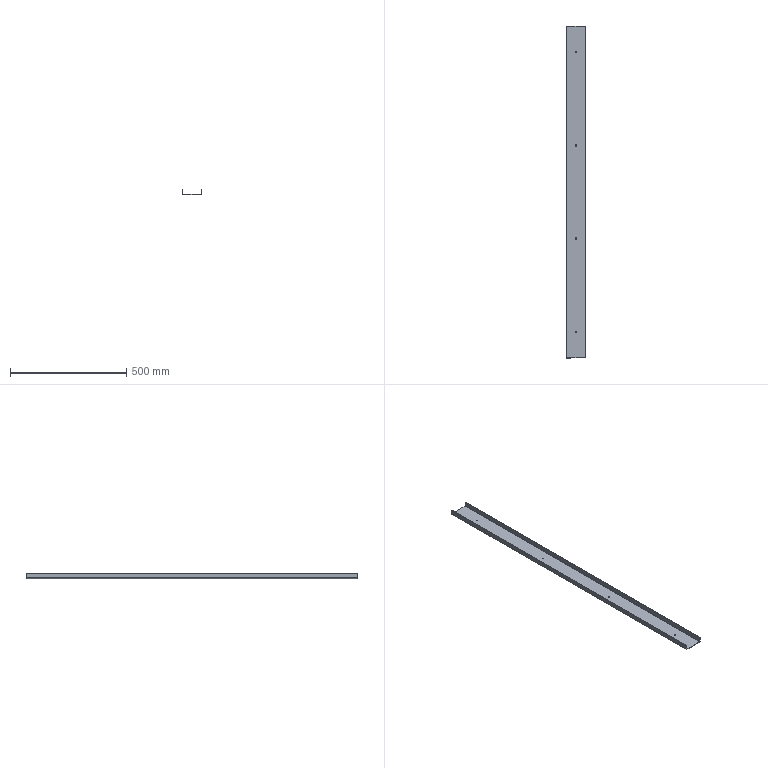Part | SolidWorks | features EdgeFlange 1, Fillet 1, FlatPattern 1, HoleWzd 1, SMBaseFlange 1, SheetMetal 1 | 1 solid | 34 faces | box 84 x 1425 x 22 mm | volume 348918 mm3 | plane 18 | cylinder 16 | commonest cylinder face diameters 5.5 x8 10 x4 1.473 x2 5.473 x2
STEP:
#1=CARTESIAN_POINT('',(-2.75,600.,-2.));
#2=VERTEX_POINT('',#1);
#3=CARTESIAN_POINT('',(2.75,600.,-2.));
#4=VERTEX_POINT('',#3);
#5=CARTESIAN_POINT('',(0.,600.,-2.));
#6=DIRECTION('',(0.,0.,1.));
#7=DIRECTION('',(1.,0.,0.));
#8=AXIS2_PLACEMENT_3D('',#5,#6,#7);
#9=CIRCLE('',#8,2.75);
#10=EDGE_CURVE('',#2,#4,#9,.T.);
#11=ORIENTED_EDGE('',*,*,#10,.F.);
#12=CARTESIAN_POINT('',(-2.75,600.,0.));
#13=VERTEX_POINT('',#12);
#14=CARTESIAN_POINT('',(-2.75,600.,0.));
#15=DIRECTION('',(0.,0.,1.));
#16=VECTOR('',#15,1000.);
#17=LINE('',#14,#16);
#18=EDGE_CURVE('',#2,#13,#17,.T.);
#19=ORIENTED_EDGE('',*,*,#18,.T.);
#20=CARTESIAN_POINT('',(2.75,600.,0.));
#21=VERTEX_POINT('',#20);
#22=CARTESIAN_POINT('',(0.,600.,0.));
#23=DIRECTION('',(0.,0.,1.));
#24=DIRECTION('',(1.,0.,0.));
#25=AXIS2_PLACEMENT_3D('',#22,#23,#24);
#26=CIRCLE('',#25,2.75);
#27=EDGE_CURVE('',#13,#21,#26,.T.);
#28=ORIENTED_EDGE('',*,*,#27,.T.);
#29=CARTESIAN_POINT('',(2.75,600.,0.));
#30=DIRECTION('',(0.,0.,1.));
#31=VECTOR('',#30,1000.);
#32=LINE('',#29,#31);
#33=EDGE_CURVE('',#4,#21,#32,.T.);
#34=ORIENTED_EDGE('',*,*,#33,.F.);
#35=EDGE_LOOP('',(#11,#19,#28,#34));
#36=FACE_OUTER_BOUND('',#35,.T.);
#37=CARTESIAN_POINT('',(0.,600.,0.));
#38=DIRECTION('',(0.,0.,1.));
#39=DIRECTION('',(1.,0.,0.));
#40=AXIS2_PLACEMENT_3D('',#37,#38,#39);
#41=CYLINDRICAL_SURFACE('',#40,2.75);
#42=ADVANCED_FACE('',(#36),#41,.F.);
#43=CARTESIAN_POINT('',(-2.75,200.,-2.));
#44=VERTEX_POINT('',#43);
#45=CARTESIAN_POINT('',(2.75,200.,-2.));
#46=VERTEX_POINT('',#45);
#47=CARTESIAN_POINT('',(0.,200.,-2.));
#48=DIRECTION('',(0.,0.,1.));
#49=DIRECTION('',(1.,0.,0.));
#50=AXIS2_PLACEMENT_3D('',#47,#48,#49);
#51=CIRCLE('',#50,2.75);
#52=EDGE_CURVE('',#44,#46,#51,.T.);
#53=ORIENTED_EDGE('',*,*,#52,.F.);
#54=CARTESIAN_POINT('',(-2.75,200.,0.));
#55=VERTEX_POINT('',#54);
#56=CARTESIAN_POINT('',(-2.75,200.,0.));
#57=DIRECTION('',(0.,0.,1.));
#58=VECTOR('',#57,1000.);
#59=LINE('',#56,#58);
#60=EDGE_CURVE('',#44,#55,#59,.T.);
#61=ORIENTED_EDGE('',*,*,#60,.T.);
#62=CARTESIAN_POINT('',(2.75,200.,0.));
#63=VERTEX_POINT('',#62);
#64=CARTESIAN_POINT('',(0.,200.,0.));
#65=DIRECTION('',(0.,0.,1.));
#66=DIRECTION('',(1.,0.,0.));
#67=AXIS2_PLACEMENT_3D('',#64,#65,#66);
#68=CIRCLE('',#67,2.75);
#69=EDGE_CURVE('',#55,#63,#68,.T.);
#70=ORIENTED_EDGE('',*,*,#69,.T.);
#71=CARTESIAN_POINT('',(2.75,200.,0.));
#72=DIRECTION('',(0.,0.,1.));
#73=VECTOR('',#72,1000.);
#74=LINE('',#71,#73);
#75=EDGE_CURVE('',#46,#63,#74,.T.);
#76=ORIENTED_EDGE('',*,*,#75,.F.);
#77=EDGE_LOOP('',(#53,#61,#70,#76));
#78=FACE_OUTER_BOUND('',#77,.T.);
#79=CARTESIAN_POINT('',(0.,200.,0.));
#80=DIRECTION('',(0.,0.,1.));
#81=DIRECTION('',(1.,0.,0.));
#82=AXIS2_PLACEMENT_3D('',#79,#80,#81);
#83=CYLINDRICAL_SURFACE('',#82,2.75);
#84=ADVANCED_FACE('',(#78),#83,.F.);
#85=CARTESIAN_POINT('',(-2.75,-200.,-2.));
#86=VERTEX_POINT('',#85);
#87=CARTESIAN_POINT('',(2.75,-200.,-2.));
#88=VERTEX_POINT('',#87);
#89=CARTESIAN_POINT('',(0.,-200.,-2.));
#90=DIRECTION('',(0.,0.,1.));
#91=DIRECTION('',(1.,0.,0.));
#92=AXIS2_PLACEMENT_3D('',#89,#90,#91);
#93=CIRCLE('',#92,2.75);
#94=EDGE_CURVE('',#86,#88,#93,.T.);
#95=ORIENTED_EDGE('',*,*,#94,.F.);
#96=CARTESIAN_POINT('',(-2.75,-200.,0.));
#97=VERTEX_POINT('',#96);
#98=CARTESIAN_POINT('',(-2.75,-200.,0.));
#99=DIRECTION('',(0.,0.,1.));
#100=VECTOR('',#99,1000.);
#101=LINE('',#98,#100);
#102=EDGE_CURVE('',#86,#97,#101,.T.);
#103=ORIENTED_EDGE('',*,*,#102,.T.);
#104=CARTESIAN_POINT('',(2.75,-200.,0.));
#105=VERTEX_POINT('',#104);
#106=CARTESIAN_POINT('',(0.,-200.,0.));
#107=DIRECTION('',(0.,0.,1.));
#108=DIRECTION('',(1.,0.,0.));
#109=AXIS2_PLACEMENT_3D('',#106,#107,#108);
#110=CIRCLE('',#109,2.75);
#111=EDGE_CURVE('',#97,#105,#110,.T.);
#112=ORIENTED_EDGE('',*,*,#111,.T.);
#113=CARTESIAN_POINT('',(2.75,-200.,0.));
#114=DIRECTION('',(0.,0.,1.));
#115=VECTOR('',#114,1000.);
#116=LINE('',#113,#115);
#117=EDGE_CURVE('',#88,#105,#116,.T.);
#118=ORIENTED_EDGE('',*,*,#117,.F.);
#119=EDGE_LOOP('',(#95,#103,#112,#118));
#120=FACE_OUTER_BOUND('',#119,.T.);
#121=CARTESIAN_POINT('',(0.,-200.,0.));
#122=DIRECTION('',(0.,0.,1.));
#123=DIRECTION('',(1.,0.,0.));
#124=AXIS2_PLACEMENT_3D('',#121,#122,#123);
#125=CYLINDRICAL_SURFACE('',#124,2.75);
#126=ADVANCED_FACE('',(#120),#125,.F.);
#127=CARTESIAN_POINT('',(-2.75,-600.,-2.));
#128=VERTEX_POINT('',#127);
#129=CARTESIAN_POINT('',(2.75,-600.,-2.));
#130=VERTEX_POINT('',#129);
#131=CARTESIAN_POINT('',(0.,-600.,-2.));
#132=DIRECTION('',(0.,0.,1.));
#133=DIRECTION('',(1.,0.,0.));
#134=AXIS2_PLACEMENT_3D('',#131,#132,#133);
#135=CIRCLE('',#134,2.75);
#136=EDGE_CURVE('',#128,#130,#135,.T.);
#137=ORIENTED_EDGE('',*,*,#136,.F.);
#138=CARTESIAN_POINT('',(-2.75,-600.,0.));
#139=VERTEX_POINT('',#138);
#140=CARTESIAN_POINT('',(-2.75,-600.,0.));
#141=DIRECTION('',(0.,0.,1.));
#142=VECTOR('',#141,1000.);
#143=LINE('',#140,#142);
#144=EDGE_CURVE('',#128,#139,#143,.T.);
#145=ORIENTED_EDGE('',*,*,#144,.T.);
#146=CARTESIAN_POINT('',(2.75,-600.,0.));
#147=VERTEX_POINT('',#146);
#148=CARTESIAN_POINT('',(0.,-600.,0.));
#149=DIRECTION('',(0.,0.,1.));
#150=DIRECTION('',(1.,0.,0.));
#151=AXIS2_PLACEMENT_3D('',#148,#149,#150);
#152=CIRCLE('',#151,2.75);
#153=EDGE_CURVE('',#139,#147,#152,.T.);
#154=ORIENTED_EDGE('',*,*,#153,.T.);
#155=CARTESIAN_POINT('',(2.75,-600.,0.));
#156=DIRECTION('',(0.,0.,1.));
#157=VECTOR('',#156,1000.);
#158=LINE('',#155,#157);
#159=EDGE_CURVE('',#130,#147,#158,.T.);
#160=ORIENTED_EDGE('',*,*,#159,.F.);
#161=EDGE_LOOP('',(#137,#145,#154,#160));
#162=FACE_OUTER_BOUND('',#161,.T.);
#163=CARTESIAN_POINT('',(0.,-600.,0.));
#164=DIRECTION('',(0.,0.,1.));
#165=DIRECTION('',(1.,0.,0.));
#166=AXIS2_PLACEMENT_3D('',#163,#164,#165);
#167=CYLINDRICAL_SURFACE('',#166,2.75);
#168=ADVANCED_FACE('',(#162),#167,.F.);
#169=CARTESIAN_POINT('',(0.,600.,-2.));
#170=DIRECTION('',(0.,0.,1.));
#171=DIRECTION('',(1.,0.,0.));
#172=AXIS2_PLACEMENT_3D('',#169,#170,#171);
#173=CIRCLE('',#172,2.75);
#174=EDGE_CURVE('',#4,#2,#173,.T.);
#175=ORIENTED_EDGE('',*,*,#174,.T.);
#176=ORIENTED_EDGE('',*,*,#10,.T.);
#177=EDGE_LOOP('',(#175,#176));
#178=FACE_BOUND('',#177,.T.);
#179=CARTESIAN_POINT('',(0.,200.,-2.));
#180=DIRECTION('',(0.,0.,1.));
#181=DIRECTION('',(1.,0.,0.));
#182=AXIS2_PLACEMENT_3D('',#179,#180,#181);
#183=CIRCLE('',#182,2.75);
#184=EDGE_CURVE('',#46,#44,#183,.T.);
#185=ORIENTED_EDGE('',*,*,#184,.T.);
#186=ORIENTED_EDGE('',*,*,#52,.T.);
#187=EDGE_LOOP('',(#185,#186));
#188=FACE_BOUND('',#187,.T.);
#189=CARTESIAN_POINT('',(0.,-200.,-2.));
#190=DIRECTION('',(0.,0.,1.));
#191=DIRECTION('',(1.,0.,0.));
#192=AXIS2_PLACEMENT_3D('',#189,#190,#191);
#193=CIRCLE('',#192,2.75);
#194=EDGE_CURVE('',#88,#86,#193,.T.);
#195=ORIENTED_EDGE('',*,*,#194,.T.);
#196=ORIENTED_EDGE('',*,*,#94,.T.);
#197=EDGE_LOOP('',(#195,#196));
#198=FACE_BOUND('',#197,.T.);
#199=CARTESIAN_POINT('',(0.,-600.,-2.));
#200=DIRECTION('',(0.,0.,1.));
#201=DIRECTION('',(1.,0.,0.));
#202=AXIS2_PLACEMENT_3D('',#199,#200,#201);
#203=CIRCLE('',#202,2.75);
#204=EDGE_CURVE('',#130,#128,#203,.T.);
#205=ORIENTED_EDGE('',*,*,#204,.T.);
#206=ORIENTED_EDGE('',*,*,#136,.T.);
#207=EDGE_LOOP('',(#205,#206));
#208=FACE_BOUND('',#207,.T.);
#209=CARTESIAN_POINT('',(-39.263,-712.5,-2.));
#210=VERTEX_POINT('',#209);
#211=CARTESIAN_POINT('',(-39.263,712.5,-2.));
#212=VERTEX_POINT('',#211);
#213=CARTESIAN_POINT('',(-39.263,-712.5,-2.));
#214=DIRECTION('',(0.,1.,0.));
#215=VECTOR('',#214,1000.);
#216=LINE('',#213,#215);
#217=EDGE_CURVE('',#210,#212,#216,.T.);
#218=ORIENTED_EDGE('',*,*,#217,.T.);
#219=CARTESIAN_POINT('',(39.263,712.5,-2.));
#220=VERTEX_POINT('',#219);
#221=CARTESIAN_POINT('',(-42.,712.5,-2.));
#222=DIRECTION('',(-1.,0.,0.));
#223=VECTOR('',#222,1000.);
#224=LINE('',#221,#223);
#225=EDGE_CURVE('',#220,#212,#224,.T.);
#226=ORIENTED_EDGE('',*,*,#225,.F.);
#227=CARTESIAN_POINT('',(39.263,-712.5,-2.));
#228=VERTEX_POINT('',#227);
#229=CARTESIAN_POINT('',(39.263,712.5,-2.));
#230=DIRECTION('',(0.,-1.,0.));
#231=VECTOR('',#230,1000.);
#232=LINE('',#229,#231);
#233=EDGE_CURVE('',#220,#228,#232,.T.);
#234=ORIENTED_EDGE('',*,*,#233,.T.);
#235=CARTESIAN_POINT('',(-42.,-712.5,-2.));
#236=DIRECTION('',(1.,0.,0.));
#237=VECTOR('',#236,1000.);
#238=LINE('',#235,#237);
#239=EDGE_CURVE('',#210,#228,#238,.T.);
#240=ORIENTED_EDGE('',*,*,#239,.F.);
#241=EDGE_LOOP('',(#218,#226,#234,#240));
#242=FACE_OUTER_BOUND('',#241,.T.);
#243=CARTESIAN_POINT('',(0.,0.,-2.));
#244=DIRECTION('',(0.,0.,1.));
#245=DIRECTION('',(1.,0.,0.));
#246=AXIS2_PLACEMENT_3D('',#243,#244,#245);
#247=PLANE('',#246);
#248=ADVANCED_FACE('',(#178,#188,#198,#208,#242),#247,.F.);
#249=CARTESIAN_POINT('',(0.,600.,0.));
#250=DIRECTION('',(0.,0.,1.));
#251=DIRECTION('',(1.,0.,0.));
#252=AXIS2_PLACEMENT_3D('',#249,#250,#251);
#253=CIRCLE('',#252,2.75);
#254=EDGE_CURVE('',#21,#13,#253,.T.);
#255=ORIENTED_EDGE('',*,*,#254,.F.);
#256=ORIENTED_EDGE('',*,*,#27,.F.);
#257=EDGE_LOOP('',(#255,#256));
#258=FACE_BOUND('',#257,.T.);
#259=CARTESIAN_POINT('',(0.,200.,0.));
#260=DIRECTION('',(0.,0.,1.));
#261=DIRECTION('',(1.,0.,0.));
#262=AXIS2_PLACEMENT_3D('',#259,#260,#261);
#263=CIRCLE('',#262,2.75);
#264=EDGE_CURVE('',#63,#55,#263,.T.);
#265=ORIENTED_EDGE('',*,*,#264,.F.);
#266=ORIENTED_EDGE('',*,*,#69,.F.);
#267=EDGE_LOOP('',(#265,#266));
#268=FACE_BOUND('',#267,.T.);
#269=CARTESIAN_POINT('',(0.,-200.,0.));
#270=DIRECTION('',(0.,0.,1.));
#271=DIRECTION('',(1.,0.,0.));
#272=AXIS2_PLACEMENT_3D('',#269,#270,#271);
#273=CIRCLE('',#272,2.75);
#274=EDGE_CURVE('',#105,#97,#273,.T.);
#275=ORIENTED_EDGE('',*,*,#274,.F.);
#276=ORIENTED_EDGE('',*,*,#111,.F.);
#277=EDGE_LOOP('',(#275,#276));
#278=FACE_BOUND('',#277,.T.);
#279=CARTESIAN_POINT('',(0.,-600.,0.));
#280=DIRECTION('',(0.,0.,1.));
#281=DIRECTION('',(1.,0.,0.));
#282=AXIS2_PLACEMENT_3D('',#279,#280,#281);
#283=CIRCLE('',#282,2.75);
#284=EDGE_CURVE('',#147,#139,#283,.T.);
#285=ORIENTED_EDGE('',*,*,#284,.F.);
#286=ORIENTED_EDGE('',*,*,#153,.F.);
#287=EDGE_LOOP('',(#285,#286));
#288=FACE_BOUND('',#287,.T.);
#289=CARTESIAN_POINT('',(39.263,712.5,0.));
#290=VERTEX_POINT('',#289);
#291=CARTESIAN_POINT('',(-39.263,712.5,0.));
#292=VERTEX_POINT('',#291);
#293=CARTESIAN_POINT('',(-42.,712.5,0.));
#294=DIRECTION('',(-1.,0.,0.));
#295=VECTOR('',#294,1000.);
#296=LINE('',#293,#295);
#297=EDGE_CURVE('',#290,#292,#296,.T.);
#298=ORIENTED_EDGE('',*,*,#297,.T.);
#299=CARTESIAN_POINT('',(-39.263,-712.5,0.));
#300=VERTEX_POINT('',#299);
#301=CARTESIAN_POINT('',(-39.263,-712.5,0.));
#302=DIRECTION('',(0.,1.,0.));
#303=VECTOR('',#302,1000.);
#304=LINE('',#301,#303);
#305=EDGE_CURVE('',#300,#292,#304,.T.);
#306=ORIENTED_EDGE('',*,*,#305,.F.);
#307=CARTESIAN_POINT('',(39.263,-712.5,0.));
#308=VERTEX_POINT('',#307);
#309=CARTESIAN_POINT('',(-42.,-712.5,0.));
#310=DIRECTION('',(1.,0.,0.));
#311=VECTOR('',#310,1000.);
#312=LINE('',#309,#311);
#313=EDGE_CURVE('',#300,#308,#312,.T.);
#314=ORIENTED_EDGE('',*,*,#313,.T.);
#315=CARTESIAN_POINT('',(39.263,712.5,0.));
#316=DIRECTION('',(0.,-1.,0.));
#317=VECTOR('',#316,1000.);
#318=LINE('',#315,#317);
#319=EDGE_CURVE('',#290,#308,#318,.T.);
#320=ORIENTED_EDGE('',*,*,#319,.F.);
#321=EDGE_LOOP('',(#298,#306,#314,#320));
#322=FACE_OUTER_BOUND('',#321,.T.);
#323=CARTESIAN_POINT('',(0.,0.,0.));
#324=DIRECTION('',(0.,0.,1.));
#325=DIRECTION('',(1.,0.,0.));
#326=AXIS2_PLACEMENT_3D('',#323,#324,#325);
#327=PLANE('',#326);
#328=ADVANCED_FACE('',(#258,#268,#278,#288,#322),#327,.T.);
#329=ORIENTED_EDGE('',*,*,#313,.F.);
#330=CARTESIAN_POINT('',(-39.263,-712.5,0.));
#331=DIRECTION('',(0.,0.,-1.));
#332=VECTOR('',#331,1000.);
#333=LINE('',#330,#332);
#334=EDGE_CURVE('',#300,#210,#333,.T.);
#335=ORIENTED_EDGE('',*,*,#334,.T.);
#336=ORIENTED_EDGE('',*,*,#239,.T.);
#337=CARTESIAN_POINT('',(39.263,-712.5,0.));
#338=DIRECTION('',(0.,0.,-1.));
#339=VECTOR('',#338,1000.);
#340=LINE('',#337,#339);
#341=EDGE_CURVE('',#308,#228,#340,.T.);
#342=ORIENTED_EDGE('',*,*,#341,.F.);
#343=EDGE_LOOP('',(#329,#335,#336,#342));
#344=FACE_OUTER_BOUND('',#343,.T.);
#345=CARTESIAN_POINT('',(-42.,-712.5,-2.));
#346=DIRECTION('',(0.,-1.,0.));
#347=DIRECTION('',(0.,0.,-1.));
#348=AXIS2_PLACEMENT_3D('',#345,#346,#347);
#349=PLANE('',#348);
#350=ADVANCED_FACE('',(#344),#349,.T.);
#351=CARTESIAN_POINT('',(-39.263,712.5,0.));
#352=DIRECTION('',(0.,0.,-1.));
#353=VECTOR('',#352,1000.);
#354=LINE('',#351,#353);
#355=EDGE_CURVE('',#292,#212,#354,.T.);
#356=ORIENTED_EDGE('',*,*,#355,.F.);
#357=ORIENTED_EDGE('',*,*,#297,.F.);
#358=CARTESIAN_POINT('',(39.263,712.5,0.));
#359=DIRECTION('',(0.,0.,-1.));
#360=VECTOR('',#359,1000.);
#361=LINE('',#358,#360);
#362=EDGE_CURVE('',#290,#220,#361,.T.);
#363=ORIENTED_EDGE('',*,*,#362,.T.);
#364=ORIENTED_EDGE('',*,*,#225,.T.);
#365=EDGE_LOOP('',(#356,#357,#363,#364));
#366=FACE_OUTER_BOUND('',#365,.T.);
#367=CARTESIAN_POINT('',(-42.,712.5,-2.));
#368=DIRECTION('',(0.,1.,0.));
#369=DIRECTION('',(0.,0.,1.));
#370=AXIS2_PLACEMENT_3D('',#367,#368,#369);
#371=PLANE('',#370);
#372=ADVANCED_FACE('',(#366),#371,.T.);
#373=CARTESIAN_POINT('',(40.,-712.5,0.7366));
#374=VERTEX_POINT('',#373);
#375=CARTESIAN_POINT('',(42.,-712.5,0.7366));
#376=VERTEX_POINT('',#375);
#377=CARTESIAN_POINT('',(42.,-712.5,0.7366));
#378=DIRECTION('',(1.,0.,0.));
#379=VECTOR('',#378,1000.);
#380=LINE('',#377,#379);
#381=EDGE_CURVE('',#374,#376,#380,.T.);
#382=ORIENTED_EDGE('',*,*,#381,.F.);
#383=CARTESIAN_POINT('',(39.263,-712.5,0.7366));
#384=DIRECTION('',(0.,-1.,0.));
#385=DIRECTION('',(0.,0.,1.));
#386=AXIS2_PLACEMENT_3D('',#383,#384,#385);
#387=CIRCLE('',#386,0.7366);
#388=EDGE_CURVE('',#308,#374,#387,.T.);
#389=ORIENTED_EDGE('',*,*,#388,.F.);
#390=ORIENTED_EDGE('',*,*,#341,.T.);
#391=CARTESIAN_POINT('',(39.263,-712.5,0.7366));
#392=DIRECTION('',(0.,-1.,0.));
#393=DIRECTION('',(0.,0.,1.));
#394=AXIS2_PLACEMENT_3D('',#391,#392,#393);
#395=CIRCLE('',#394,2.737);
#396=EDGE_CURVE('',#228,#376,#395,.T.);
#397=ORIENTED_EDGE('',*,*,#396,.T.);
#398=EDGE_LOOP('',(#382,#389,#390,#397));
#399=FACE_OUTER_BOUND('',#398,.T.);
#400=CARTESIAN_POINT('',(39.263,-712.5,0.7366));
#401=DIRECTION('',(0.,-1.,0.));
#402=DIRECTION('',(0.,0.,-1.));
#403=AXIS2_PLACEMENT_3D('',#400,#401,#402);
#404=PLANE('',#403);
#405=ADVANCED_FACE('',(#399),#404,.T.);
#406=CARTESIAN_POINT('',(40.,712.5,0.7366));
#407=VERTEX_POINT('',#406);
#408=CARTESIAN_POINT('',(39.263,712.5,0.7366));
#409=DIRECTION('',(0.,1.,0.));
#410=DIRECTION('',(0.,0.,1.));
#411=AXIS2_PLACEMENT_3D('',#408,#409,#410);
#412=CIRCLE('',#411,0.7366);
#413=EDGE_CURVE('',#407,#290,#412,.T.);
#414=ORIENTED_EDGE('',*,*,#413,.F.);
#415=CARTESIAN_POINT('',(42.,712.5,0.7366));
#416=VERTEX_POINT('',#415);
#417=CARTESIAN_POINT('',(40.,712.5,0.7366));
#418=DIRECTION('',(1.,0.,0.));
#419=VECTOR('',#418,1000.);
#420=LINE('',#417,#419);
#421=EDGE_CURVE('',#407,#416,#420,.T.);
#422=ORIENTED_EDGE('',*,*,#421,.T.);
#423=CARTESIAN_POINT('',(39.263,712.5,0.7366));
#424=DIRECTION('',(0.,1.,0.));
#425=DIRECTION('',(0.,0.,1.));
#426=AXIS2_PLACEMENT_3D('',#423,#424,#425);
#427=CIRCLE('',#426,2.737);
#428=EDGE_CURVE('',#416,#220,#427,.T.);
#429=ORIENTED_EDGE('',*,*,#428,.T.);
#430=ORIENTED_EDGE('',*,*,#362,.F.);
#431=EDGE_LOOP('',(#414,#422,#429,#430));
#432=FACE_OUTER_BOUND('',#431,.T.);
#433=CARTESIAN_POINT('',(39.263,712.5,0.7366));
#434=DIRECTION('',(0.,-1.,0.));
#435=DIRECTION('',(0.,0.,-1.));
#436=AXIS2_PLACEMENT_3D('',#433,#434,#435);
#437=PLANE('',#436);
#438=ADVANCED_FACE('',(#432),#437,.F.);
#439=ORIENTED_EDGE('',*,*,#233,.F.);
#440=ORIENTED_EDGE('',*,*,#428,.F.);
#441=CARTESIAN_POINT('',(42.,-712.5,0.7366));
#442=DIRECTION('',(0.,-1.,0.));
#443=VECTOR('',#442,1000.);
#444=LINE('',#441,#443);
#445=EDGE_CURVE('',#416,#376,#444,.T.);
#446=ORIENTED_EDGE('',*,*,#445,.T.);
#447=ORIENTED_EDGE('',*,*,#396,.F.);
#448=EDGE_LOOP('',(#439,#440,#446,#447));
#449=FACE_OUTER_BOUND('',#448,.T.);
#450=CARTESIAN_POINT('',(39.263,712.5,0.7366));
#451=DIRECTION('',(0.,1.,0.));
#452=DIRECTION('',(1.,0.,0.));
#453=AXIS2_PLACEMENT_3D('',#450,#451,#452);
#454=CYLINDRICAL_SURFACE('',#453,2.737);
#455=ADVANCED_FACE('',(#449),#454,.T.);
#456=ORIENTED_EDGE('',*,*,#319,.T.);
#457=ORIENTED_EDGE('',*,*,#388,.T.);
#458=CARTESIAN_POINT('',(40.,-712.5,0.7366));
#459=DIRECTION('',(0.,1.,0.));
#460=VECTOR('',#459,1000.);
#461=LINE('',#458,#460);
#462=EDGE_CURVE('',#374,#407,#461,.T.);
#463=ORIENTED_EDGE('',*,*,#462,.T.);
#464=ORIENTED_EDGE('',*,*,#413,.T.);
#465=EDGE_LOOP('',(#456,#457,#463,#464));
#466=FACE_OUTER_BOUND('',#465,.T.);
#467=CARTESIAN_POINT('',(39.263,712.5,0.7366));
#468=DIRECTION('',(0.,1.,0.));
#469=DIRECTION('',(1.,0.,0.));
#470=AXIS2_PLACEMENT_3D('',#467,#468,#469);
#471=CYLINDRICAL_SURFACE('',#470,0.7366);
#472=ADVANCED_FACE('',(#466),#471,.F.);
#473=CARTESIAN_POINT('',(40.,712.5,15.));
#474=VERTEX_POINT('',#473);
#475=CARTESIAN_POINT('',(40.,712.5,20.));
#476=DIRECTION('',(0.,0.,1.));
#477=VECTOR('',#476,1000.);
#478=LINE('',#475,#477);
#479=EDGE_CURVE('',#407,#474,#478,.T.);
#480=ORIENTED_EDGE('',*,*,#479,.T.);
#481=CARTESIAN_POINT('',(42.,712.5,15.));
#482=VERTEX_POINT('',#481);
#483=CARTESIAN_POINT('',(42.,712.5,15.));
#484=DIRECTION('',(1.,0.,0.));
#485=VECTOR('',#484,1000.);
#486=LINE('',#483,#485);
#487=EDGE_CURVE('',#474,#482,#486,.T.);
#488=ORIENTED_EDGE('',*,*,#487,.T.);
#489=CARTESIAN_POINT('',(42.,712.5,0.));
#490=DIRECTION('',(0.,0.,1.));
#491=VECTOR('',#490,1000.);
#492=LINE('',#489,#491);
#493=EDGE_CURVE('',#416,#482,#492,.T.);
#494=ORIENTED_EDGE('',*,*,#493,.F.);
#495=ORIENTED_EDGE('',*,*,#421,.F.);
#496=EDGE_LOOP('',(#480,#488,#494,#495));
#497=FACE_OUTER_BOUND('',#496,.T.);
#498=CARTESIAN_POINT('',(42.,712.5,20.));
#499=DIRECTION('',(0.,-1.,0.));
#500=DIRECTION('',(0.,0.,-1.));
#501=AXIS2_PLACEMENT_3D('',#498,#499,#500);
#502=PLANE('',#501);
#503=ADVANCED_FACE('',(#497),#502,.F.);
#504=CARTESIAN_POINT('',(42.,-712.5,15.));
#505=VERTEX_POINT('',#504);
#506=CARTESIAN_POINT('',(42.,-712.5,0.));
#507=DIRECTION('',(0.,0.,-1.));
#508=VECTOR('',#507,1000.);
#509=LINE('',#506,#508);
#510=EDGE_CURVE('',#505,#376,#509,.T.);
#511=ORIENTED_EDGE('',*,*,#510,.F.);
#512=CARTESIAN_POINT('',(40.,-712.5,15.));
#513=VERTEX_POINT('',#512);
#514=CARTESIAN_POINT('',(42.,-712.5,15.));
#515=DIRECTION('',(-1.,0.,0.));
#516=VECTOR('',#515,1000.);
#517=LINE('',#514,#516);
#518=EDGE_CURVE('',#505,#513,#517,.T.);
#519=ORIENTED_EDGE('',*,*,#518,.T.);
#520=CARTESIAN_POINT('',(40.,-712.5,0.));
#521=DIRECTION('',(0.,0.,-1.));
#522=VECTOR('',#521,1000.);
#523=LINE('',#520,#522);
#524=EDGE_CURVE('',#513,#374,#523,.T.);
#525=ORIENTED_EDGE('',*,*,#524,.T.);
#526=ORIENTED_EDGE('',*,*,#381,.T.);
#527=EDGE_LOOP('',(#511,#519,#525,#526));
#528=FACE_OUTER_BOUND('',#527,.T.);
#529=CARTESIAN_POINT('',(42.,-712.5,0.));
#530=DIRECTION('',(0.,1.,0.));
#531=DIRECTION('',(0.,0.,1.));
#532=AXIS2_PLACEMENT_3D('',#529,#530,#531);
#533=PLANE('',#532);
#534=ADVANCED_FACE('',(#528),#533,.F.);
#535=CARTESIAN_POINT('',(42.,707.5,20.));
#536=VERTEX_POINT('',#535);
#537=CARTESIAN_POINT('',(42.,-707.5,20.));
#538=VERTEX_POINT('',#537);
#539=CARTESIAN_POINT('',(42.,0.,20.));
#540=DIRECTION('',(0.,-1.,0.));
#541=VECTOR('',#540,1000.);
#542=LINE('',#539,#541);
#543=EDGE_CURVE('',#536,#538,#542,.T.);
#544=ORIENTED_EDGE('',*,*,#543,.T.);
#545=CARTESIAN_POINT('',(42.,-707.5,15.));
#546=DIRECTION('',(1.,0.,0.));
#547=DIRECTION('',(0.,0.,1.));
#548=AXIS2_PLACEMENT_3D('',#545,#546,#547);
#549=CIRCLE('',#548,5.);
#550=EDGE_CURVE('',#538,#505,#549,.T.);
#551=ORIENTED_EDGE('',*,*,#550,.T.);
#552=ORIENTED_EDGE('',*,*,#510,.T.);
#553=ORIENTED_EDGE('',*,*,#445,.F.);
#554=ORIENTED_EDGE('',*,*,#493,.T.);
#555=CARTESIAN_POINT('',(42.,707.5,15.));
#556=DIRECTION('',(1.,0.,0.));
#557=DIRECTION('',(0.,0.,1.));
#558=AXIS2_PLACEMENT_3D('',#555,#556,#557);
#559=CIRCLE('',#558,5.);
#560=EDGE_CURVE('',#482,#536,#559,.T.);
#561=ORIENTED_EDGE('',*,*,#560,.T.);
#562=EDGE_LOOP('',(#544,#551,#552,#553,#554,#561));
#563=FACE_OUTER_BOUND('',#562,.T.);
#564=CARTESIAN_POINT('',(42.,0.,0.));
#565=DIRECTION('',(-1.,0.,0.));
#566=DIRECTION('',(0.,0.,1.));
#567=AXIS2_PLACEMENT_3D('',#564,#565,#566);
#568=PLANE('',#567);
#569=ADVANCED_FACE('',(#563),#568,.F.);
#570=ORIENTED_EDGE('',*,*,#524,.F.);
#571=CARTESIAN_POINT('',(40.,-707.5,20.));
#572=VERTEX_POINT('',#571);
#573=CARTESIAN_POINT('',(40.,-707.5,15.));
#574=DIRECTION('',(-1.,0.,0.));
#575=DIRECTION('',(0.,0.,1.));
#576=AXIS2_PLACEMENT_3D('',#573,#574,#575);
#577=CIRCLE('',#576,5.);
#578=EDGE_CURVE('',#513,#572,#577,.T.);
#579=ORIENTED_EDGE('',*,*,#578,.T.);
#580=CARTESIAN_POINT('',(40.,707.5,20.));
#581=VERTEX_POINT('',#580);
#582=CARTESIAN_POINT('',(40.,-712.5,20.));
#583=DIRECTION('',(0.,-1.,0.));
#584=VECTOR('',#583,1000.);
#585=LINE('',#582,#584);
#586=EDGE_CURVE('',#581,#572,#585,.T.);
#587=ORIENTED_EDGE('',*,*,#586,.F.);
#588=CARTESIAN_POINT('',(40.,707.5,15.));
#589=DIRECTION('',(-1.,0.,0.));
#590=DIRECTION('',(0.,0.,1.));
#591=AXIS2_PLACEMENT_3D('',#588,#589,#590);
#592=CIRCLE('',#591,5.);
#593=EDGE_CURVE('',#581,#474,#592,.T.);
#594=ORIENTED_EDGE('',*,*,#593,.T.);
#595=ORIENTED_EDGE('',*,*,#479,.F.);
#596=ORIENTED_EDGE('',*,*,#462,.F.);
#597=EDGE_LOOP('',(#570,#579,#587,#594,#595,#596));
#598=FACE_OUTER_BOUND('',#597,.T.);
#599=CARTESIAN_POINT('',(40.,0.,0.));
#600=DIRECTION('',(-1.,0.,0.));
#601=DIRECTION('',(0.,0.,1.));
#602=AXIS2_PLACEMENT_3D('',#599,#600,#601);
#603=PLANE('',#602);
#604=ADVANCED_FACE('',(#598),#603,.T.);
#605=ORIENTED_EDGE('',*,*,#586,.T.);
#606=CARTESIAN_POINT('',(42.,-707.5,20.));
#607=DIRECTION('',(1.,0.,0.));
#608=VECTOR('',#607,1000.);
#609=LINE('',#606,#608);
#610=EDGE_CURVE('',#572,#538,#609,.T.);
#611=ORIENTED_EDGE('',*,*,#610,.T.);
#612=ORIENTED_EDGE('',*,*,#543,.F.);
#613=CARTESIAN_POINT('',(42.,707.5,20.));
#614=DIRECTION('',(-1.,0.,0.));
#615=VECTOR('',#614,1000.);
#616=LINE('',#613,#615);
#617=EDGE_CURVE('',#536,#581,#616,.T.);
#618=ORIENTED_EDGE('',*,*,#617,.T.);
#619=EDGE_LOOP('',(#605,#611,#612,#618));
#620=FACE_OUTER_BOUND('',#619,.T.);
#621=CARTESIAN_POINT('',(42.,-712.5,20.));
#622=DIRECTION('',(0.,0.,-1.));
#623=DIRECTION('',(-1.,0.,0.));
#624=AXIS2_PLACEMENT_3D('',#621,#622,#623);
#625=PLANE('',#624);
#626=ADVANCED_FACE('',(#620),#625,.F.);
#627=CARTESIAN_POINT('',(-40.,712.5,0.7366));
#628=VERTEX_POINT('',#627);
#629=CARTESIAN_POINT('',(-42.,712.5,0.7366));
#630=VERTEX_POINT('',#629);
#631=CARTESIAN_POINT('',(-42.,712.5,0.7366));
#632=DIRECTION('',(-1.,0.,0.));
#633=VECTOR('',#632,1000.);
#634=LINE('',#631,#633);
#635=EDGE_CURVE('',#628,#630,#634,.T.);
#636=ORIENTED_EDGE('',*,*,#635,.F.);
#637=CARTESIAN_POINT('',(-39.263,712.5,0.7366));
#638=DIRECTION('',(0.,1.,0.));
#639=DIRECTION('',(0.,0.,-1.));
#640=AXIS2_PLACEMENT_3D('',#637,#638,#639);
#641=CIRCLE('',#640,0.7366);
#642=EDGE_CURVE('',#292,#628,#641,.T.);
#643=ORIENTED_EDGE('',*,*,#642,.F.);
#644=ORIENTED_EDGE('',*,*,#355,.T.);
#645=CARTESIAN_POINT('',(-39.263,712.5,0.7366));
#646=DIRECTION('',(0.,1.,0.));
#647=DIRECTION('',(0.,0.,-1.));
#648=AXIS2_PLACEMENT_3D('',#645,#646,#647);
#649=CIRCLE('',#648,2.737);
#650=EDGE_CURVE('',#212,#630,#649,.T.);
#651=ORIENTED_EDGE('',*,*,#650,.T.);
#652=EDGE_LOOP('',(#636,#643,#644,#651));
#653=FACE_OUTER_BOUND('',#652,.T.);
#654=CARTESIAN_POINT('',(-39.263,712.5,0.7366));
#655=DIRECTION('',(0.,1.,0.));
#656=DIRECTION('',(0.,0.,1.));
#657=AXIS2_PLACEMENT_3D('',#654,#655,#656);
#658=PLANE('',#657);
#659=ADVANCED_FACE('',(#653),#658,.T.);
#660=CARTESIAN_POINT('',(-40.,-712.5,0.7366));
#661=VERTEX_POINT('',#660);
#662=CARTESIAN_POINT('',(-39.263,-712.5,0.7366));
#663=DIRECTION('',(0.,-1.,0.));
#664=DIRECTION('',(0.,0.,-1.));
#665=AXIS2_PLACEMENT_3D('',#662,#663,#664);
#666=CIRCLE('',#665,0.7366);
#667=EDGE_CURVE('',#661,#300,#666,.T.);
#668=ORIENTED_EDGE('',*,*,#667,.F.);
#669=CARTESIAN_POINT('',(-42.,-712.5,0.7366));
#670=VERTEX_POINT('',#669);
#671=CARTESIAN_POINT('',(-40.,-712.5,0.7366));
#672=DIRECTION('',(-1.,0.,0.));
#673=VECTOR('',#672,1000.);
#674=LINE('',#671,#673);
#675=EDGE_CURVE('',#661,#670,#674,.T.);
#676=ORIENTED_EDGE('',*,*,#675,.T.);
#677=CARTESIAN_POINT('',(-39.263,-712.5,0.7366));
#678=DIRECTION('',(0.,-1.,0.));
#679=DIRECTION('',(0.,0.,-1.));
#680=AXIS2_PLACEMENT_3D('',#677,#678,#679);
#681=CIRCLE('',#680,2.737);
#682=EDGE_CURVE('',#670,#210,#681,.T.);
#683=ORIENTED_EDGE('',*,*,#682,.T.);
#684=ORIENTED_EDGE('',*,*,#334,.F.);
#685=EDGE_LOOP('',(#668,#676,#683,#684));
#686=FACE_OUTER_BOUND('',#685,.T.);
#687=CARTESIAN_POINT('',(-39.263,-712.5,0.7366));
#688=DIRECTION('',(0.,1.,0.));
#689=DIRECTION('',(0.,0.,1.));
#690=AXIS2_PLACEMENT_3D('',#687,#688,#689);
#691=PLANE('',#690);
#692=ADVANCED_FACE('',(#686),#691,.F.);
#693=ORIENTED_EDGE('',*,*,#217,.F.);
#694=ORIENTED_EDGE('',*,*,#682,.F.);
#695=CARTESIAN_POINT('',(-42.,712.5,0.7366));
#696=DIRECTION('',(0.,1.,0.));
#697=VECTOR('',#696,1000.);
#698=LINE('',#695,#697);
#699=EDGE_CURVE('',#670,#630,#698,.T.);
#700=ORIENTED_EDGE('',*,*,#699,.T.);
#701=ORIENTED_EDGE('',*,*,#650,.F.);
#702=EDGE_LOOP('',(#693,#694,#700,#701));
#703=FACE_OUTER_BOUND('',#702,.T.);
#704=CARTESIAN_POINT('',(-39.263,-712.5,0.7366));
#705=DIRECTION('',(0.,-1.,0.));
#706=DIRECTION('',(-1.,0.,0.));
#707=AXIS2_PLACEMENT_3D('',#704,#705,#706);
#708=CYLINDRICAL_SURFACE('',#707,2.737);
#709=ADVANCED_FACE('',(#703),#708,.T.);
#710=ORIENTED_EDGE('',*,*,#305,.T.);
#711=ORIENTED_EDGE('',*,*,#642,.T.);
#712=CARTESIAN_POINT('',(-40.,712.5,0.7366));
#713=DIRECTION('',(0.,-1.,0.));
#714=VECTOR('',#713,1000.);
#715=LINE('',#712,#714);
#716=EDGE_CURVE('',#628,#661,#715,.T.);
#717=ORIENTED_EDGE('',*,*,#716,.T.);
#718=ORIENTED_EDGE('',*,*,#667,.T.);
#719=EDGE_LOOP('',(#710,#711,#717,#718));
#720=FACE_OUTER_BOUND('',#719,.T.);
#721=CARTESIAN_POINT('',(-39.263,-712.5,0.7366));
#722=DIRECTION('',(0.,-1.,0.));
#723=DIRECTION('',(-1.,0.,0.));
#724=AXIS2_PLACEMENT_3D('',#721,#722,#723);
#725=CYLINDRICAL_SURFACE('',#724,0.7366);
#726=ADVANCED_FACE('',(#720),#725,.F.);
#727=CARTESIAN_POINT('',(-42.,712.5,15.));
#728=VERTEX_POINT('',#727);
#729=CARTESIAN_POINT('',(-42.,712.5,0.));
#730=DIRECTION('',(0.,0.,-1.));
#731=VECTOR('',#730,1000.);
#732=LINE('',#729,#731);
#733=EDGE_CURVE('',#728,#630,#732,.T.);
#734=ORIENTED_EDGE('',*,*,#733,.F.);
#735=CARTESIAN_POINT('',(-40.,712.5,15.));
#736=VERTEX_POINT('',#735);
#737=CARTESIAN_POINT('',(-42.,712.5,15.));
#738=DIRECTION('',(1.,0.,0.));
#739=VECTOR('',#738,1000.);
#740=LINE('',#737,#739);
#741=EDGE_CURVE('',#728,#736,#740,.T.);
#742=ORIENTED_EDGE('',*,*,#741,.T.);
#743=CARTESIAN_POINT('',(-40.,712.5,0.));
#744=DIRECTION('',(0.,0.,-1.));
#745=VECTOR('',#744,1000.);
#746=LINE('',#743,#745);
#747=EDGE_CURVE('',#736,#628,#746,.T.);
#748=ORIENTED_EDGE('',*,*,#747,.T.);
#749=ORIENTED_EDGE('',*,*,#635,.T.);
#750=EDGE_LOOP('',(#734,#742,#748,#749));
#751=FACE_OUTER_BOUND('',#750,.T.);
#752=CARTESIAN_POINT('',(-42.,712.5,0.));
#753=DIRECTION('',(0.,-1.,0.));
#754=DIRECTION('',(0.,0.,-1.));
#755=AXIS2_PLACEMENT_3D('',#752,#753,#754);
#756=PLANE('',#755);
#757=ADVANCED_FACE('',(#751),#756,.F.);
#758=CARTESIAN_POINT('',(-40.,-712.5,15.));
#759=VERTEX_POINT('',#758);
#760=CARTESIAN_POINT('',(-40.,-712.5,20.));
#761=DIRECTION('',(0.,0.,1.));
#762=VECTOR('',#761,1000.);
#763=LINE('',#760,#762);
#764=EDGE_CURVE('',#661,#759,#763,.T.);
#765=ORIENTED_EDGE('',*,*,#764,.T.);
#766=CARTESIAN_POINT('',(-42.,-712.5,15.));
#767=VERTEX_POINT('',#766);
#768=CARTESIAN_POINT('',(-42.,-712.5,15.));
#769=DIRECTION('',(-1.,0.,0.));
#770=VECTOR('',#769,1000.);
#771=LINE('',#768,#770);
#772=EDGE_CURVE('',#759,#767,#771,.T.);
#773=ORIENTED_EDGE('',*,*,#772,.T.);
#774=CARTESIAN_POINT('',(-42.,-712.5,0.));
#775=DIRECTION('',(0.,0.,1.));
#776=VECTOR('',#775,1000.);
#777=LINE('',#774,#776);
#778=EDGE_CURVE('',#670,#767,#777,.T.);
#779=ORIENTED_EDGE('',*,*,#778,.F.);
#780=ORIENTED_EDGE('',*,*,#675,.F.);
#781=EDGE_LOOP('',(#765,#773,#779,#780));
#782=FACE_OUTER_BOUND('',#781,.T.);
#783=CARTESIAN_POINT('',(-42.,-712.5,20.));
#784=DIRECTION('',(0.,1.,0.));
#785=DIRECTION('',(0.,0.,1.));
#786=AXIS2_PLACEMENT_3D('',#783,#784,#785);
#787=PLANE('',#786);
#788=ADVANCED_FACE('',(#782),#787,.F.);
#789=ORIENTED_EDGE('',*,*,#778,.T.);
#790=CARTESIAN_POINT('',(-42.,-707.5,20.));
#791=VERTEX_POINT('',#790);
#792=CARTESIAN_POINT('',(-42.,-707.5,15.));
#793=DIRECTION('',(-1.,0.,0.));
#794=DIRECTION('',(0.,0.,-1.));
#795=AXIS2_PLACEMENT_3D('',#792,#793,#794);
#796=CIRCLE('',#795,5.);
#797=EDGE_CURVE('',#767,#791,#796,.T.);
#798=ORIENTED_EDGE('',*,*,#797,.T.);
#799=CARTESIAN_POINT('',(-42.,707.5,20.));
#800=VERTEX_POINT('',#799);
#801=CARTESIAN_POINT('',(-42.,0.,20.));
#802=DIRECTION('',(0.,1.,0.));
#803=VECTOR('',#802,1000.);
#804=LINE('',#801,#803);
#805=EDGE_CURVE('',#791,#800,#804,.T.);
#806=ORIENTED_EDGE('',*,*,#805,.T.);
#807=CARTESIAN_POINT('',(-42.,707.5,15.));
#808=DIRECTION('',(-1.,0.,0.));
#809=DIRECTION('',(0.,0.,-1.));
#810=AXIS2_PLACEMENT_3D('',#807,#808,#809);
#811=CIRCLE('',#810,5.);
#812=EDGE_CURVE('',#800,#728,#811,.T.);
#813=ORIENTED_EDGE('',*,*,#812,.T.);
#814=ORIENTED_EDGE('',*,*,#733,.T.);
#815=ORIENTED_EDGE('',*,*,#699,.F.);
#816=EDGE_LOOP('',(#789,#798,#806,#813,#814,#815));
#817=FACE_OUTER_BOUND('',#816,.T.);
#818=CARTESIAN_POINT('',(-42.,0.,0.));
#819=DIRECTION('',(1.,0.,0.));
#820=DIRECTION('',(0.,0.,-1.));
#821=AXIS2_PLACEMENT_3D('',#818,#819,#820);
#822=PLANE('',#821);
#823=ADVANCED_FACE('',(#817),#822,.F.);
#824=CARTESIAN_POINT('',(-40.,-707.5,20.));
#825=VERTEX_POINT('',#824);
#826=CARTESIAN_POINT('',(-40.,707.5,20.));
#827=VERTEX_POINT('',#826);
#828=CARTESIAN_POINT('',(-40.,712.5,20.));
#829=DIRECTION('',(0.,1.,0.));
#830=VECTOR('',#829,1000.);
#831=LINE('',#828,#830);
#832=EDGE_CURVE('',#825,#827,#831,.T.);
#833=ORIENTED_EDGE('',*,*,#832,.F.);
#834=CARTESIAN_POINT('',(-40.,-707.5,15.));
#835=DIRECTION('',(1.,0.,0.));
#836=DIRECTION('',(0.,0.,-1.));
#837=AXIS2_PLACEMENT_3D('',#834,#835,#836);
#838=CIRCLE('',#837,5.);
#839=EDGE_CURVE('',#825,#759,#838,.T.);
#840=ORIENTED_EDGE('',*,*,#839,.T.);
#841=ORIENTED_EDGE('',*,*,#764,.F.);
#842=ORIENTED_EDGE('',*,*,#716,.F.);
#843=ORIENTED_EDGE('',*,*,#747,.F.);
#844=CARTESIAN_POINT('',(-40.,707.5,15.));
#845=DIRECTION('',(1.,0.,0.));
#846=DIRECTION('',(0.,0.,-1.));
#847=AXIS2_PLACEMENT_3D('',#844,#845,#846);
#848=CIRCLE('',#847,5.);
#849=EDGE_CURVE('',#736,#827,#848,.T.);
#850=ORIENTED_EDGE('',*,*,#849,.T.);
#851=EDGE_LOOP('',(#833,#840,#841,#842,#843,#850));
#852=FACE_OUTER_BOUND('',#851,.T.);
#853=CARTESIAN_POINT('',(-40.,0.,0.));
#854=DIRECTION('',(1.,0.,0.));
#855=DIRECTION('',(0.,0.,-1.));
#856=AXIS2_PLACEMENT_3D('',#853,#854,#855);
#857=PLANE('',#856);
#858=ADVANCED_FACE('',(#852),#857,.T.);
#859=ORIENTED_EDGE('',*,*,#805,.F.);
#860=CARTESIAN_POINT('',(-42.,-707.5,20.));
#861=DIRECTION('',(1.,0.,0.));
#862=VECTOR('',#861,1000.);
#863=LINE('',#860,#862);
#864=EDGE_CURVE('',#791,#825,#863,.T.);
#865=ORIENTED_EDGE('',*,*,#864,.T.);
#866=ORIENTED_EDGE('',*,*,#832,.T.);
#867=CARTESIAN_POINT('',(-42.,707.5,20.));
#868=DIRECTION('',(-1.,0.,0.));
#869=VECTOR('',#868,1000.);
#870=LINE('',#867,#869);
#871=EDGE_CURVE('',#827,#800,#870,.T.);
#872=ORIENTED_EDGE('',*,*,#871,.T.);
#873=EDGE_LOOP('',(#859,#865,#866,#872));
#874=FACE_OUTER_BOUND('',#873,.T.);
#875=CARTESIAN_POINT('',(-42.,712.5,20.));
#876=DIRECTION('',(0.,0.,-1.));
#877=DIRECTION('',(-1.,0.,0.));
#878=AXIS2_PLACEMENT_3D('',#875,#876,#877);
#879=PLANE('',#878);
#880=ADVANCED_FACE('',(#874),#879,.F.);
#881=ORIENTED_EDGE('',*,*,#144,.F.);
#882=ORIENTED_EDGE('',*,*,#204,.F.);
#883=ORIENTED_EDGE('',*,*,#159,.T.);
#884=ORIENTED_EDGE('',*,*,#284,.T.);
#885=EDGE_LOOP('',(#881,#882,#883,#884));
#886=FACE_OUTER_BOUND('',#885,.T.);
#887=CARTESIAN_POINT('',(0.,-600.,0.));
#888=DIRECTION('',(0.,0.,1.));
#889=DIRECTION('',(1.,0.,0.));
#890=AXIS2_PLACEMENT_3D('',#887,#888,#889);
#891=CYLINDRICAL_SURFACE('',#890,2.75);
#892=ADVANCED_FACE('',(#886),#891,.F.);
#893=ORIENTED_EDGE('',*,*,#102,.F.);
#894=ORIENTED_EDGE('',*,*,#194,.F.);
#895=ORIENTED_EDGE('',*,*,#117,.T.);
#896=ORIENTED_EDGE('',*,*,#274,.T.);
#897=EDGE_LOOP('',(#893,#894,#895,#896));
#898=FACE_OUTER_BOUND('',#897,.T.);
#899=CARTESIAN_POINT('',(0.,-200.,0.));
#900=DIRECTION('',(0.,0.,1.));
#901=DIRECTION('',(1.,0.,0.));
#902=AXIS2_PLACEMENT_3D('',#899,#900,#901);
#903=CYLINDRICAL_SURFACE('',#902,2.75);
#904=ADVANCED_FACE('',(#898),#903,.F.);
#905=ORIENTED_EDGE('',*,*,#60,.F.);
#906=ORIENTED_EDGE('',*,*,#184,.F.);
#907=ORIENTED_EDGE('',*,*,#75,.T.);
#908=ORIENTED_EDGE('',*,*,#264,.T.);
#909=EDGE_LOOP('',(#905,#906,#907,#908));
#910=FACE_OUTER_BOUND('',#909,.T.);
#911=CARTESIAN_POINT('',(0.,200.,0.));
#912=DIRECTION('',(0.,0.,1.));
#913=DIRECTION('',(1.,0.,0.));
#914=AXIS2_PLACEMENT_3D('',#911,#912,#913);
#915=CYLINDRICAL_SURFACE('',#914,2.75);
#916=ADVANCED_FACE('',(#910),#915,.F.);
#917=ORIENTED_EDGE('',*,*,#18,.F.);
#918=ORIENTED_EDGE('',*,*,#174,.F.);
#919=ORIENTED_EDGE('',*,*,#33,.T.);
#920=ORIENTED_EDGE('',*,*,#254,.T.);
#921=EDGE_LOOP('',(#917,#918,#919,#920));
#922=FACE_OUTER_BOUND('',#921,.T.);
#923=CARTESIAN_POINT('',(0.,600.,0.));
#924=DIRECTION('',(0.,0.,1.));
#925=DIRECTION('',(1.,0.,0.));
#926=AXIS2_PLACEMENT_3D('',#923,#924,#925);
#927=CYLINDRICAL_SURFACE('',#926,2.75);
#928=ADVANCED_FACE('',(#922),#927,.F.);
#929=ORIENTED_EDGE('',*,*,#550,.F.);
#930=ORIENTED_EDGE('',*,*,#610,.F.);
#931=ORIENTED_EDGE('',*,*,#578,.F.);
#932=ORIENTED_EDGE('',*,*,#518,.F.);
#933=EDGE_LOOP('',(#929,#930,#931,#932));
#934=FACE_OUTER_BOUND('',#933,.T.);
#935=CARTESIAN_POINT('',(42.,-707.5,15.));
#936=DIRECTION('',(-1.,0.,0.));
#937=DIRECTION('',(0.,0.,1.));
#938=AXIS2_PLACEMENT_3D('',#935,#936,#937);
#939=CYLINDRICAL_SURFACE('',#938,5.);
#940=ADVANCED_FACE('',(#934),#939,.T.);
#941=ORIENTED_EDGE('',*,*,#797,.F.);
#942=ORIENTED_EDGE('',*,*,#772,.F.);
#943=ORIENTED_EDGE('',*,*,#839,.F.);
#944=ORIENTED_EDGE('',*,*,#864,.F.);
#945=EDGE_LOOP('',(#941,#942,#943,#944));
#946=FACE_OUTER_BOUND('',#945,.T.);
#947=CARTESIAN_POINT('',(-42.,-707.5,15.));
#948=DIRECTION('',(1.,0.,0.));
#949=DIRECTION('',(0.,0.,-1.));
#950=AXIS2_PLACEMENT_3D('',#947,#948,#949);
#951=CYLINDRICAL_SURFACE('',#950,5.);
#952=ADVANCED_FACE('',(#946),#951,.T.);
#953=ORIENTED_EDGE('',*,*,#560,.F.);
#954=ORIENTED_EDGE('',*,*,#487,.F.);
#955=ORIENTED_EDGE('',*,*,#593,.F.);
#956=ORIENTED_EDGE('',*,*,#617,.F.);
#957=EDGE_LOOP('',(#953,#954,#955,#956));
#958=FACE_OUTER_BOUND('',#957,.T.);
#959=CARTESIAN_POINT('',(42.,707.5,15.));
#960=DIRECTION('',(-1.,0.,0.));
#961=DIRECTION('',(0.,0.,1.));
#962=AXIS2_PLACEMENT_3D('',#959,#960,#961);
#963=CYLINDRICAL_SURFACE('',#962,5.);
#964=ADVANCED_FACE('',(#958),#963,.T.);
#965=ORIENTED_EDGE('',*,*,#812,.F.);
#966=ORIENTED_EDGE('',*,*,#871,.F.);
#967=ORIENTED_EDGE('',*,*,#849,.F.);
#968=ORIENTED_EDGE('',*,*,#741,.F.);
#969=EDGE_LOOP('',(#965,#966,#967,#968));
#970=FACE_OUTER_BOUND('',#969,.T.);
#971=CARTESIAN_POINT('',(-42.,707.5,15.));
#972=DIRECTION('',(1.,0.,0.));
#973=DIRECTION('',(0.,0.,-1.));
#974=AXIS2_PLACEMENT_3D('',#971,#972,#973);
#975=CYLINDRICAL_SURFACE('',#974,5.);
#976=ADVANCED_FACE('',(#970),#975,.T.);
#977=CLOSED_SHELL('',(#42,#84,#126,#168,#248,#328,#350,#372,#405,#438,#455,#472,#503,#534,#569,#604,#626,#659,#692,#709,#726,#757,#788,#823,#858,#880,#892,#904,#916,#928,#940,#952,#964,#976));
#978=MANIFOLD_SOLID_BREP('',#977);
#979=CARTESIAN_POINT('',(0.,0.,0.));
#980=DIRECTION('',(0.,0.,1.));
#981=DIRECTION('',(1.,0.,0.));
#982=AXIS2_PLACEMENT_3D('',#979,#980,#981);
#983=(LENGTH_UNIT()NAMED_UNIT(*)SI_UNIT(.MILLI.,.METRE.));
#984=UNCERTAINTY_MEASURE_WITH_UNIT(LENGTH_MEASURE(0.00001),#983,'','');
#985=(NAMED_UNIT(*)PLANE_ANGLE_UNIT()SI_UNIT($,.RADIAN.));
#986=(NAMED_UNIT(*)SI_UNIT($,.STERADIAN.)SOLID_ANGLE_UNIT());
#987=(GEOMETRIC_REPRESENTATION_CONTEXT(3)GLOBAL_UNCERTAINTY_ASSIGNED_CONTEXT((#984))GLOBAL_UNIT_ASSIGNED_CONTEXT((#983,#985,#986))REPRESENTATION_CONTEXT('',''));
#988=ADVANCED_BREP_SHAPE_REPRESENTATION('',(#978,#982),#987);